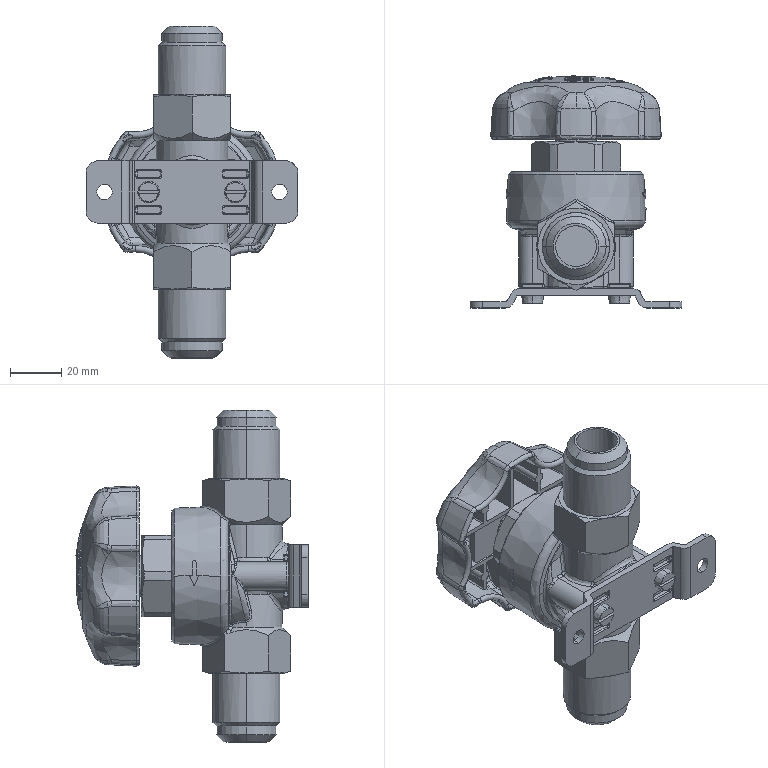Part | STEP file | BML18S | 1 solid | 1666 faces | box 83 x 90.853 x 130 mm | volume 164797 mm3 | plane 538 | cylinder 457 | spline 382 | torus 123 | sphere 89 | cone 77 | commonest cylinder face diameters 1 x55 2 x33 0.762 x32 0.504 x26 3 x13 0.5 x12